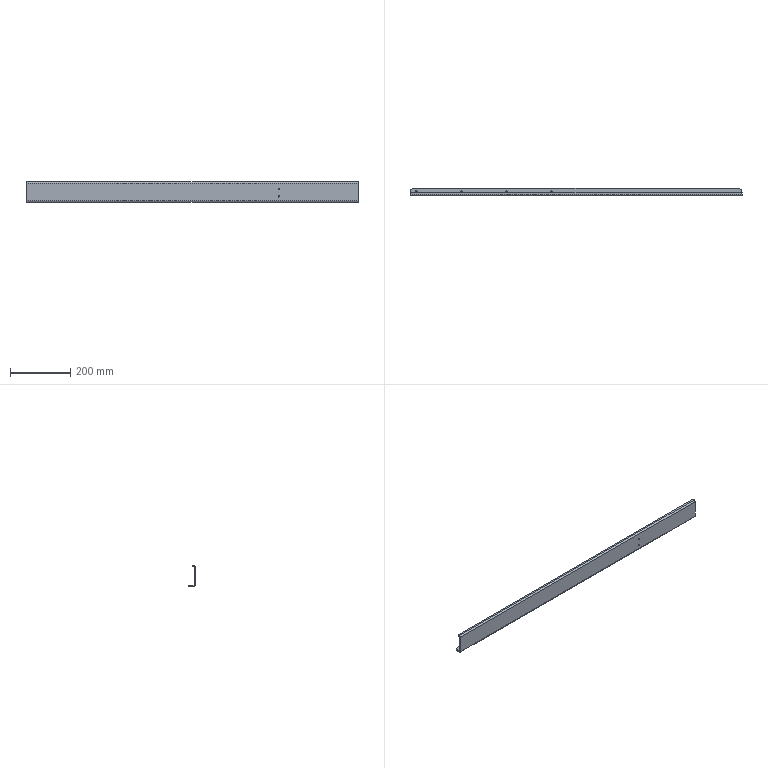Part | STEP file | drag chain fixing plate_default | 1 solid | 38 faces | box 1100 x 25 x 68 mm | volume 406508 mm3 | cylinder 20 | plane 18 | commonest cylinder face diameters 7 x8 4.2 x4 1.473 x2 9.473 x2 10 x2 30 x2